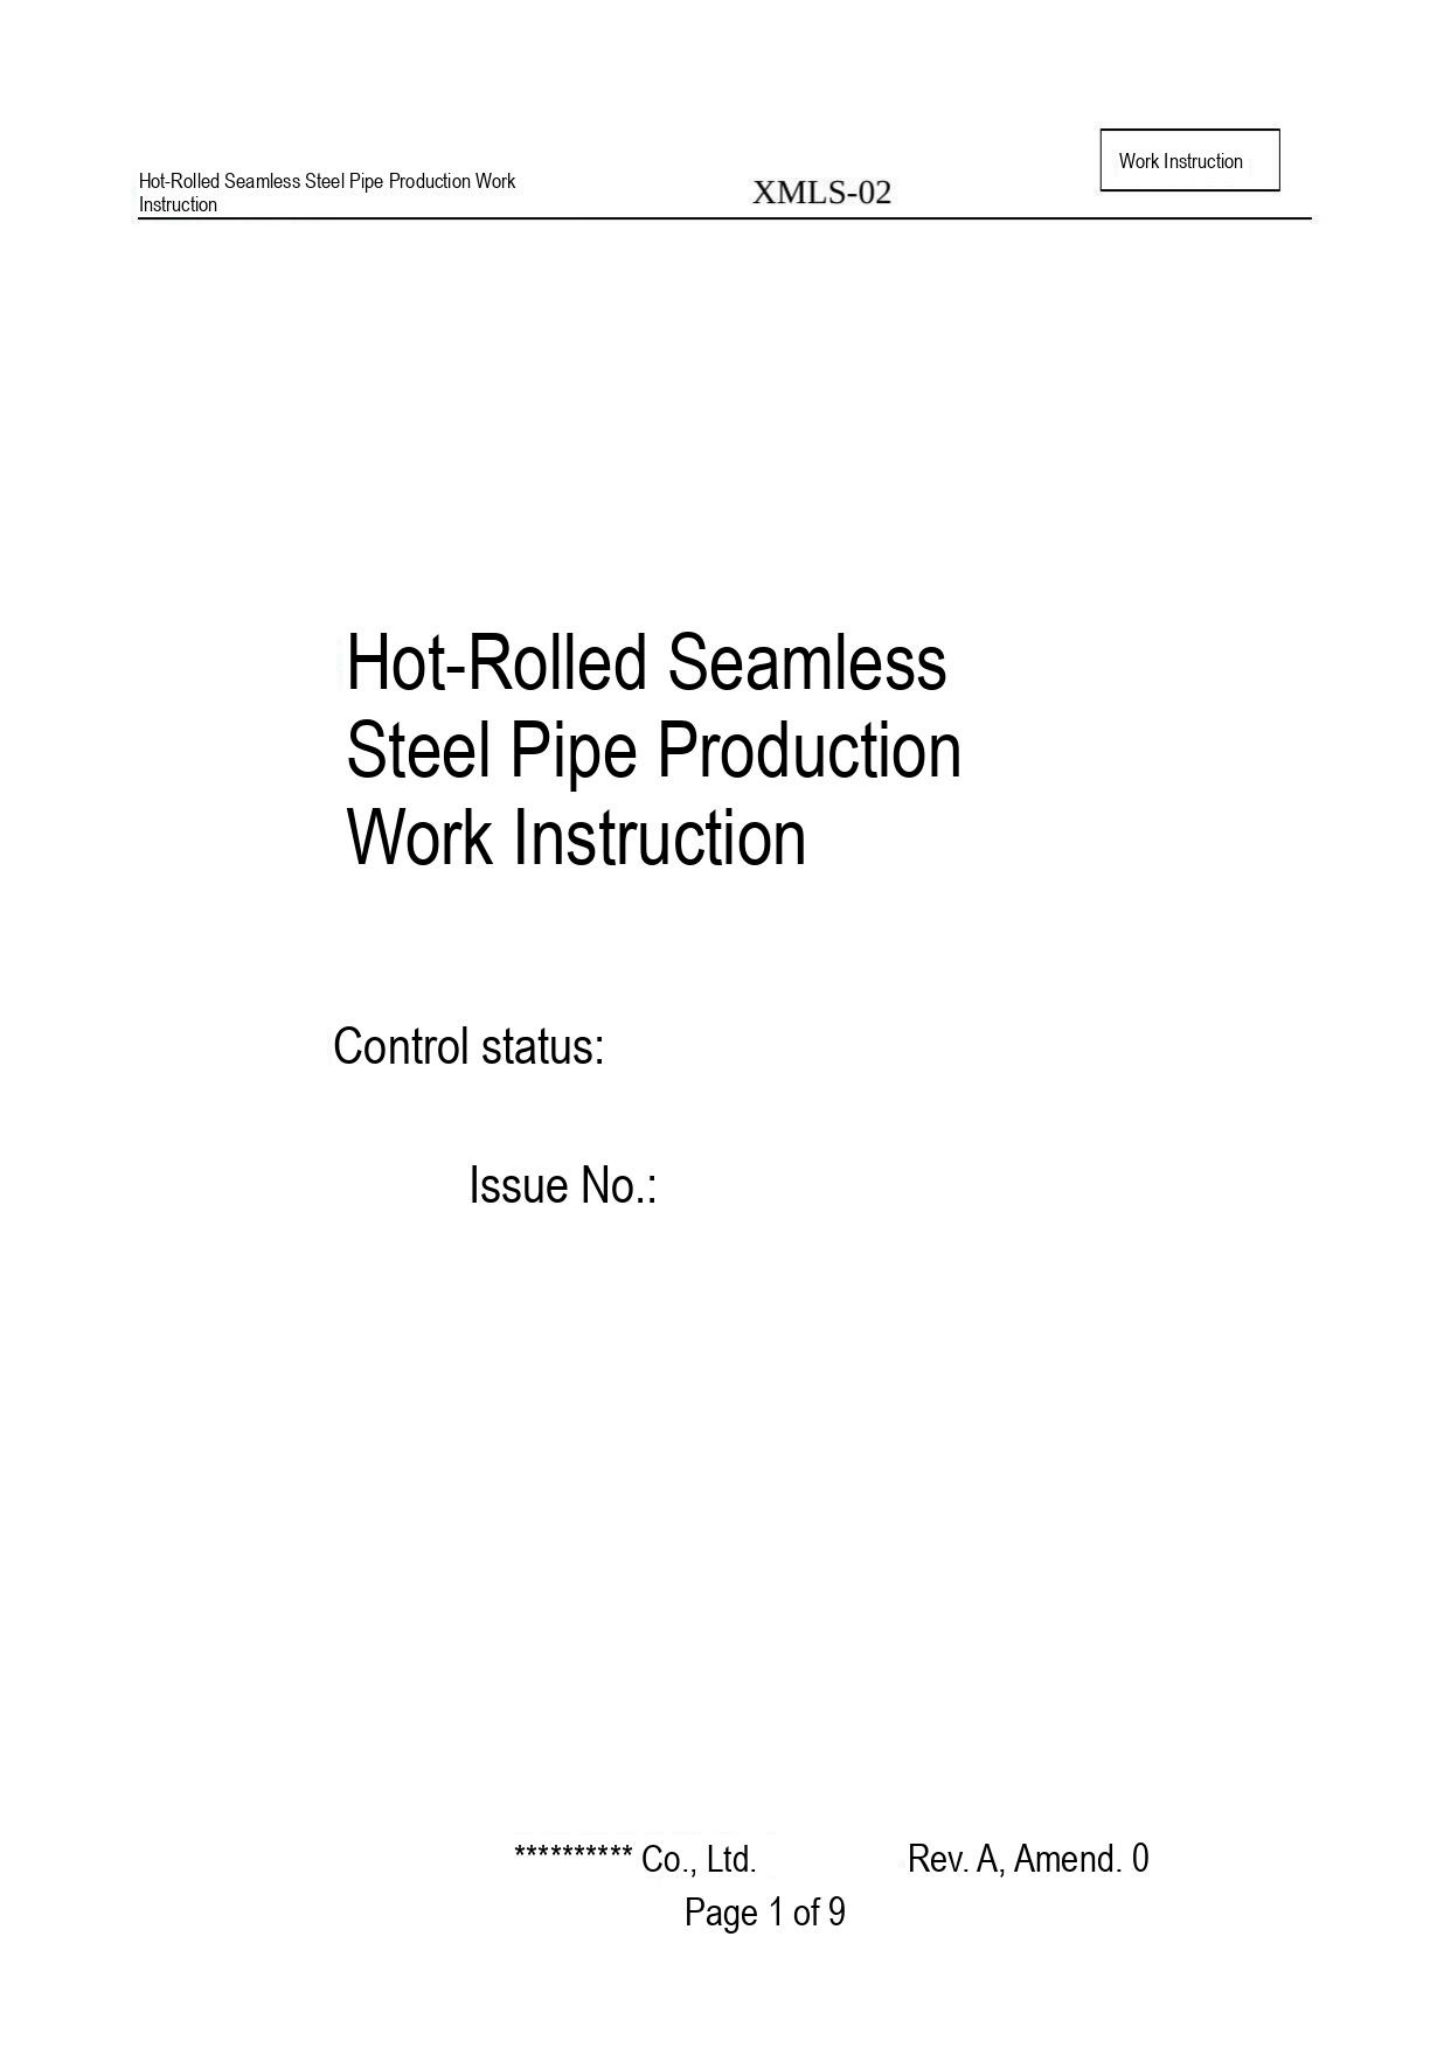Hot-Rolled Seamless Steel Pipe Production Work Instruction

XMLS-02

Work Instruction

Hot-Rolled Seamless Steel Pipe Production Work Instruction

Control status:

Issue No.:

********** Co., Ltd.

Rev. A, Amend. 0

Page 1 of 9
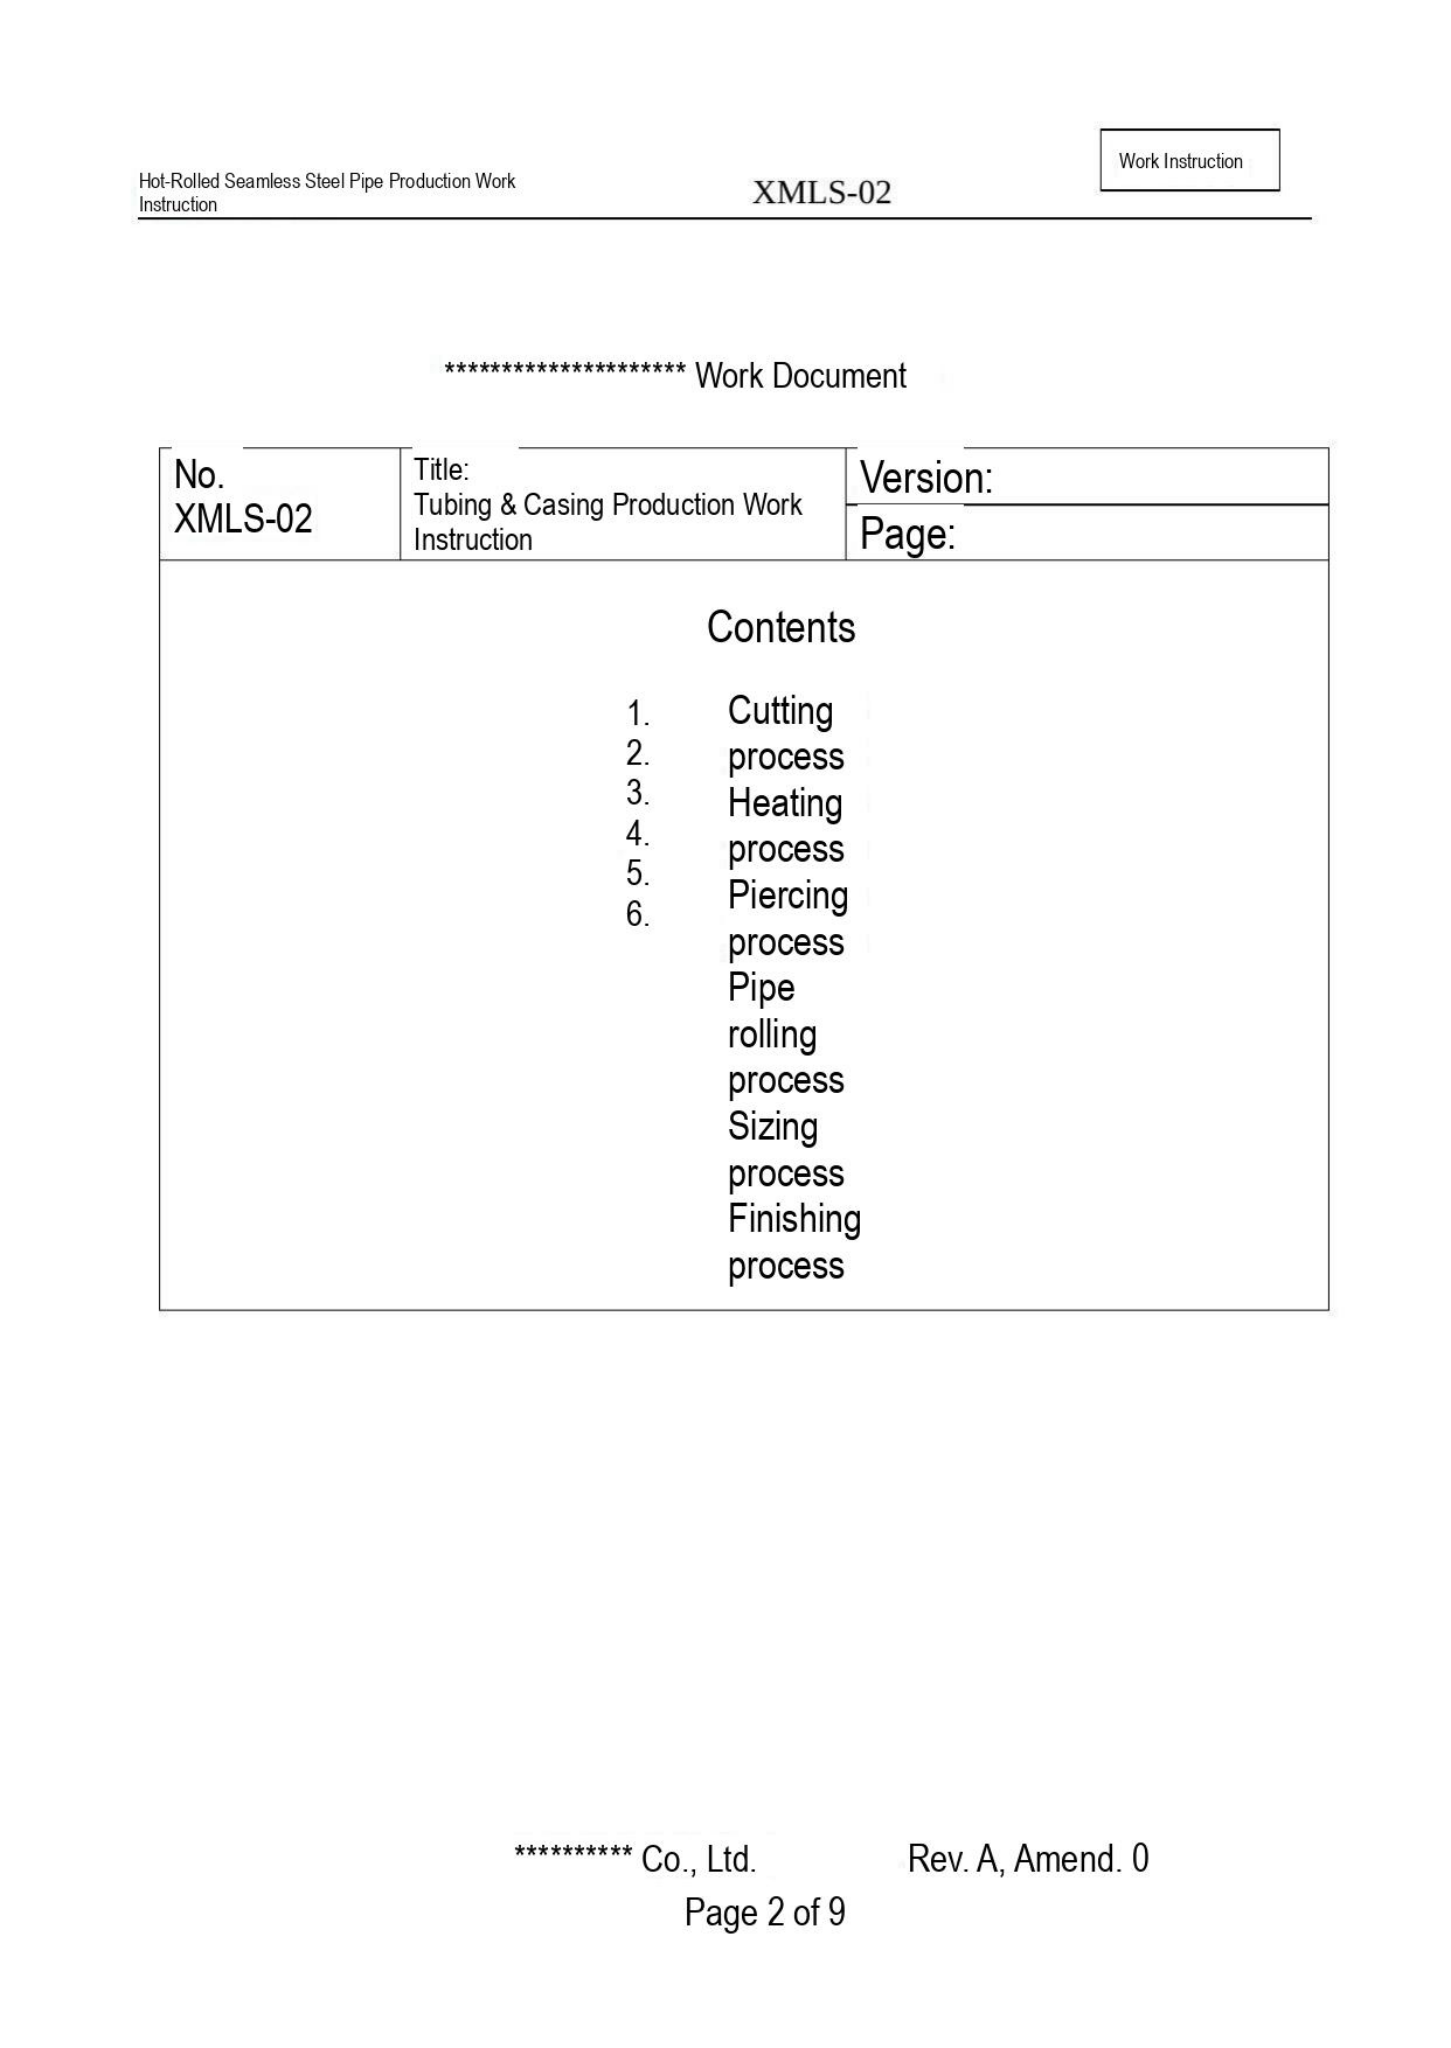Hot-Rolled Seamless Steel Pipe Production Work Instruction

XMLS-02

Work Instruction

********************* Work Document

| No. XMLS-02 | Title: Tubing & Casing Production Work Instruction | Version: |
|---|---|---|
| | | Page: |

Contents

1. Cutting process
2. Heating process
3. Piercing process
4. Pipe rolling process
5. Sizing process
6. Finishing process

********** Co., Ltd. Rev. A, Amend. 0

Page 2 of 9
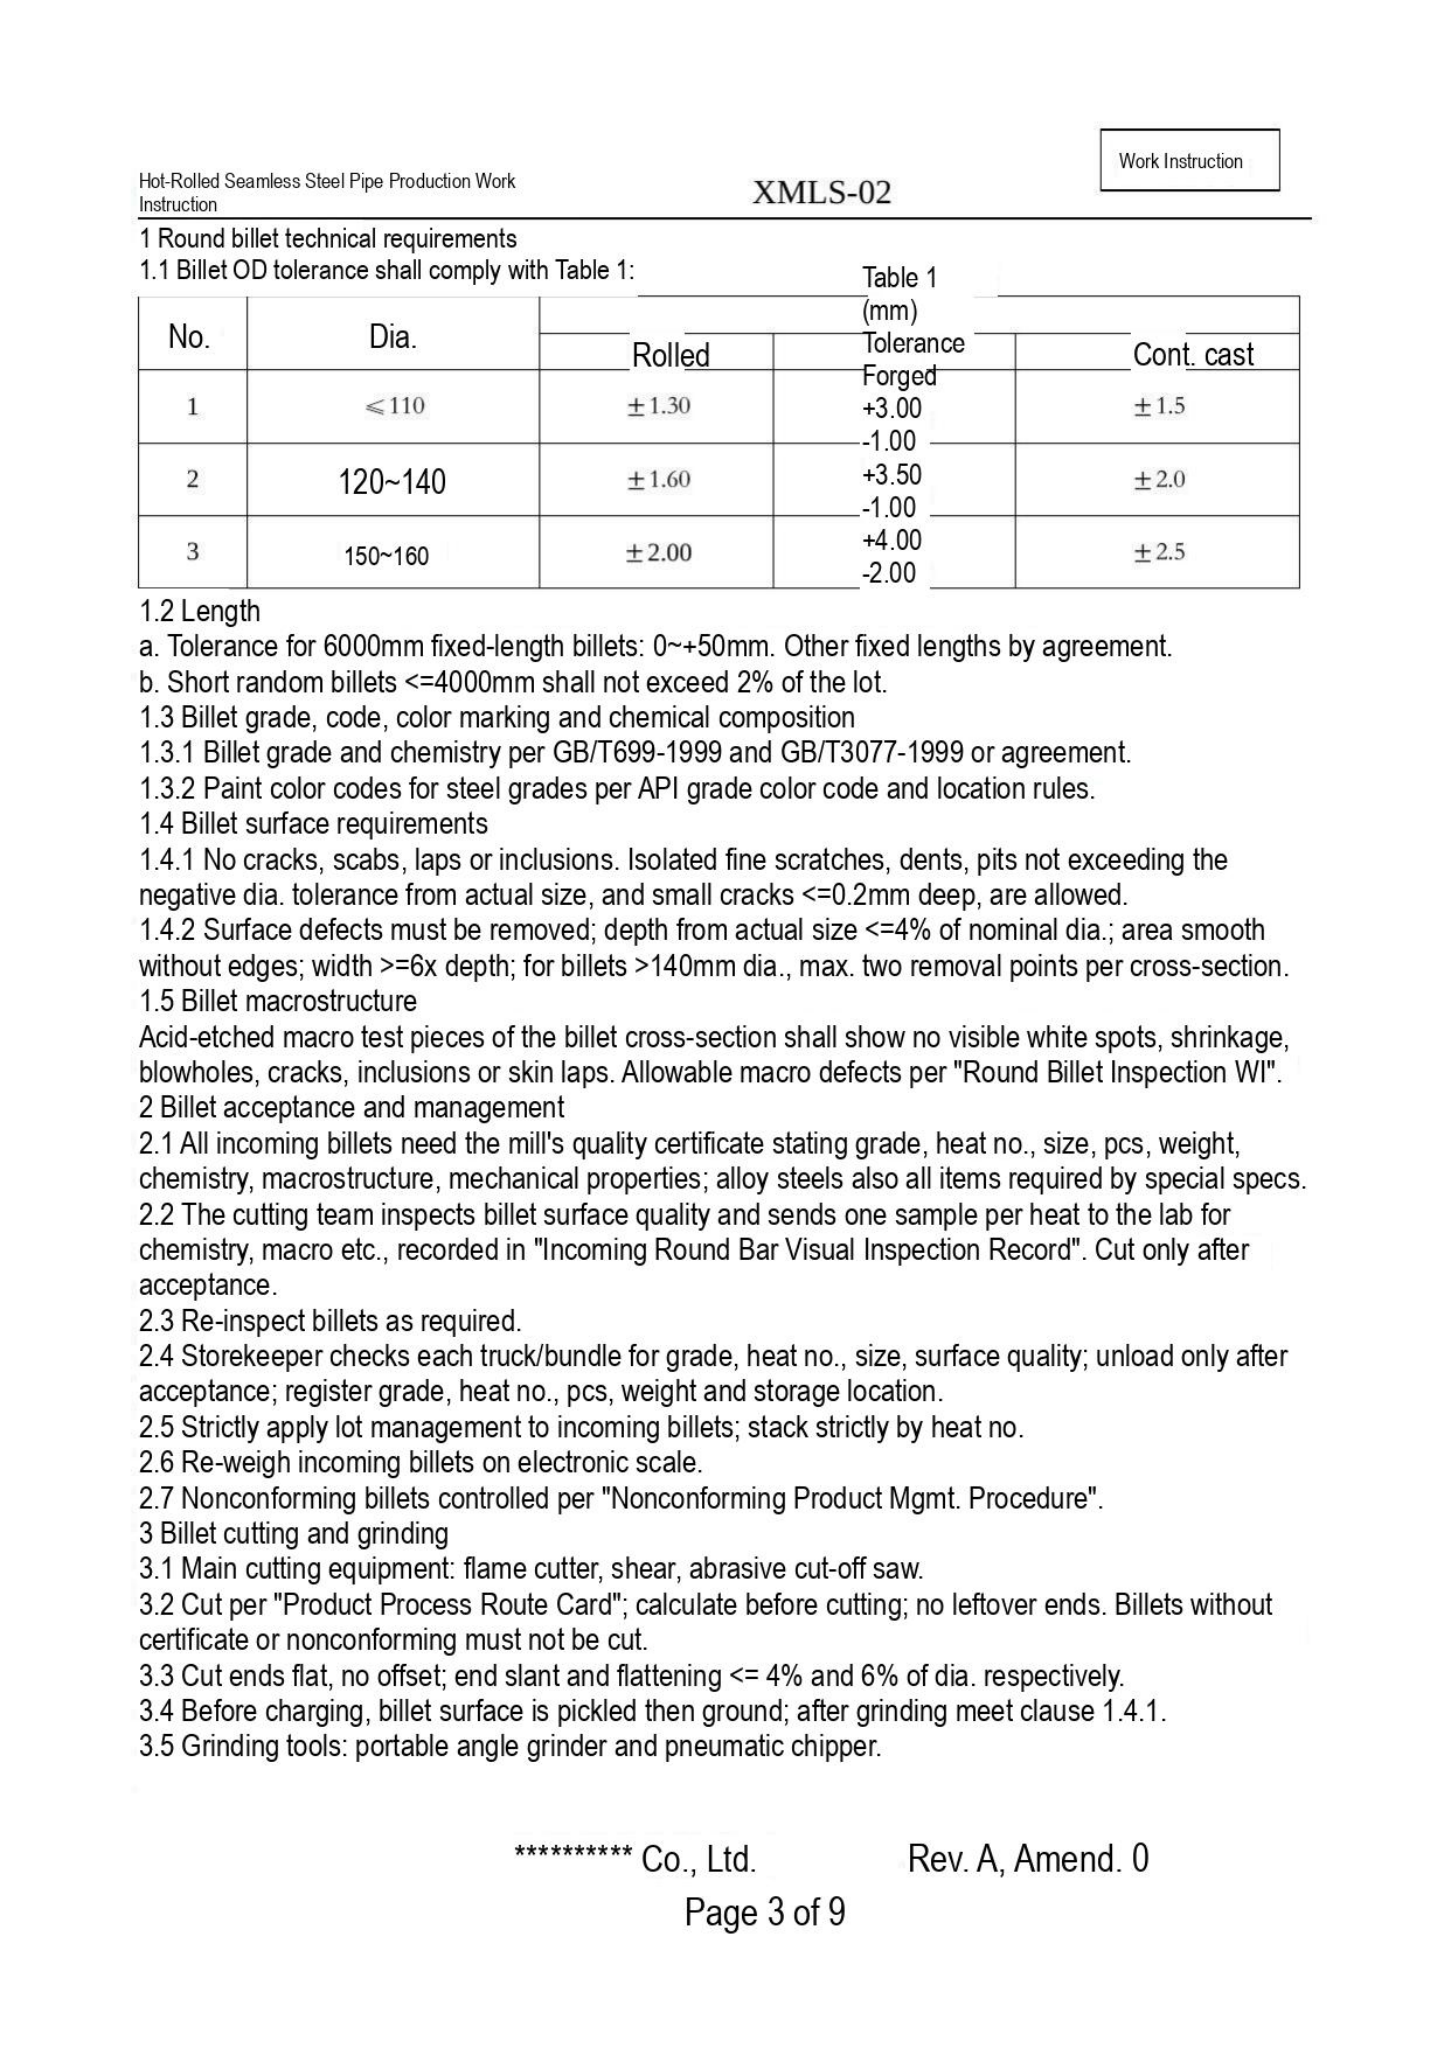Hot-Rolled Seamless Steel Pipe Production Work Instruction

XMLS-02

Work Instruction

1 Round billet technical requirements

1.1 Billet OD tolerance shall comply with Table 1:

Table 1 (mm)

| No. | Dia. | Tolerance<br>Rolled | Tolerance<br>Forged | Tolerance<br>Cont. cast |
|---|---|---|---|---|
| 1 | ≤110 | ±1.30 | +3.00<br>-1.00 | ±1.5 |
| 2 | 120~140 | ±1.60 | +3.50<br>-1.00 | ±2.0 |
| 3 | 150~160 | ±2.00 | +4.00<br>-2.00 | ±2.5 |

1.2 Length

a. Tolerance for 6000mm fixed-length billets: 0~+50mm. Other fixed lengths by agreement.

b. Short random billets <=4000mm shall not exceed 2% of the lot.

1.3 Billet grade, code, color marking and chemical composition

1.3.1 Billet grade and chemistry per GB/T699-1999 and GB/T3077-1999 or agreement.

1.3.2 Paint color codes for steel grades per API grade color code and location rules.

1.4 Billet surface requirements

1.4.1 No cracks, scabs, laps or inclusions. Isolated fine scratches, dents, pits not exceeding the negative dia. tolerance from actual size, and small cracks <=0.2mm deep, are allowed.

1.4.2 Surface defects must be removed; depth from actual size <=4% of nominal dia.; area smooth without edges; width >=6x depth; for billets >140mm dia., max. two removal points per cross-section.

1.5 Billet macrostructure

Acid-etched macro test pieces of the billet cross-section shall show no visible white spots, shrinkage, blowholes, cracks, inclusions or skin laps. Allowable macro defects per "Round Billet Inspection WI".

2 Billet acceptance and management

2.1 All incoming billets need the mill's quality certificate stating grade, heat no., size, pcs, weight, chemistry, macrostructure, mechanical properties; alloy steels also all items required by special specs.

2.2 The cutting team inspects billet surface quality and sends one sample per heat to the lab for chemistry, macro etc., recorded in "Incoming Round Bar Visual Inspection Record". Cut only after acceptance.

2.3 Re-inspect billets as required.

2.4 Storekeeper checks each truck/bundle for grade, heat no., size, surface quality; unload only after acceptance; register grade, heat no., pcs, weight and storage location.

2.5 Strictly apply lot management to incoming billets; stack strictly by heat no.

2.6 Re-weigh incoming billets on electronic scale.

2.7 Nonconforming billets controlled per "Nonconforming Product Mgmt. Procedure".

3 Billet cutting and grinding

3.1 Main cutting equipment: flame cutter, shear, abrasive cut-off saw.

3.2 Cut per "Product Process Route Card"; calculate before cutting; no leftover ends. Billets without certificate or nonconforming must not be cut.

3.3 Cut ends flat, no offset; end slant and flattening <= 4% and 6% of dia. respectively.

3.4 Before charging, billet surface is pickled then ground; after grinding meet clause 1.4.1.

3.5 Grinding tools: portable angle grinder and pneumatic chipper.

********** Co., Ltd. Rev. A, Amend. 0

Page 3 of 9
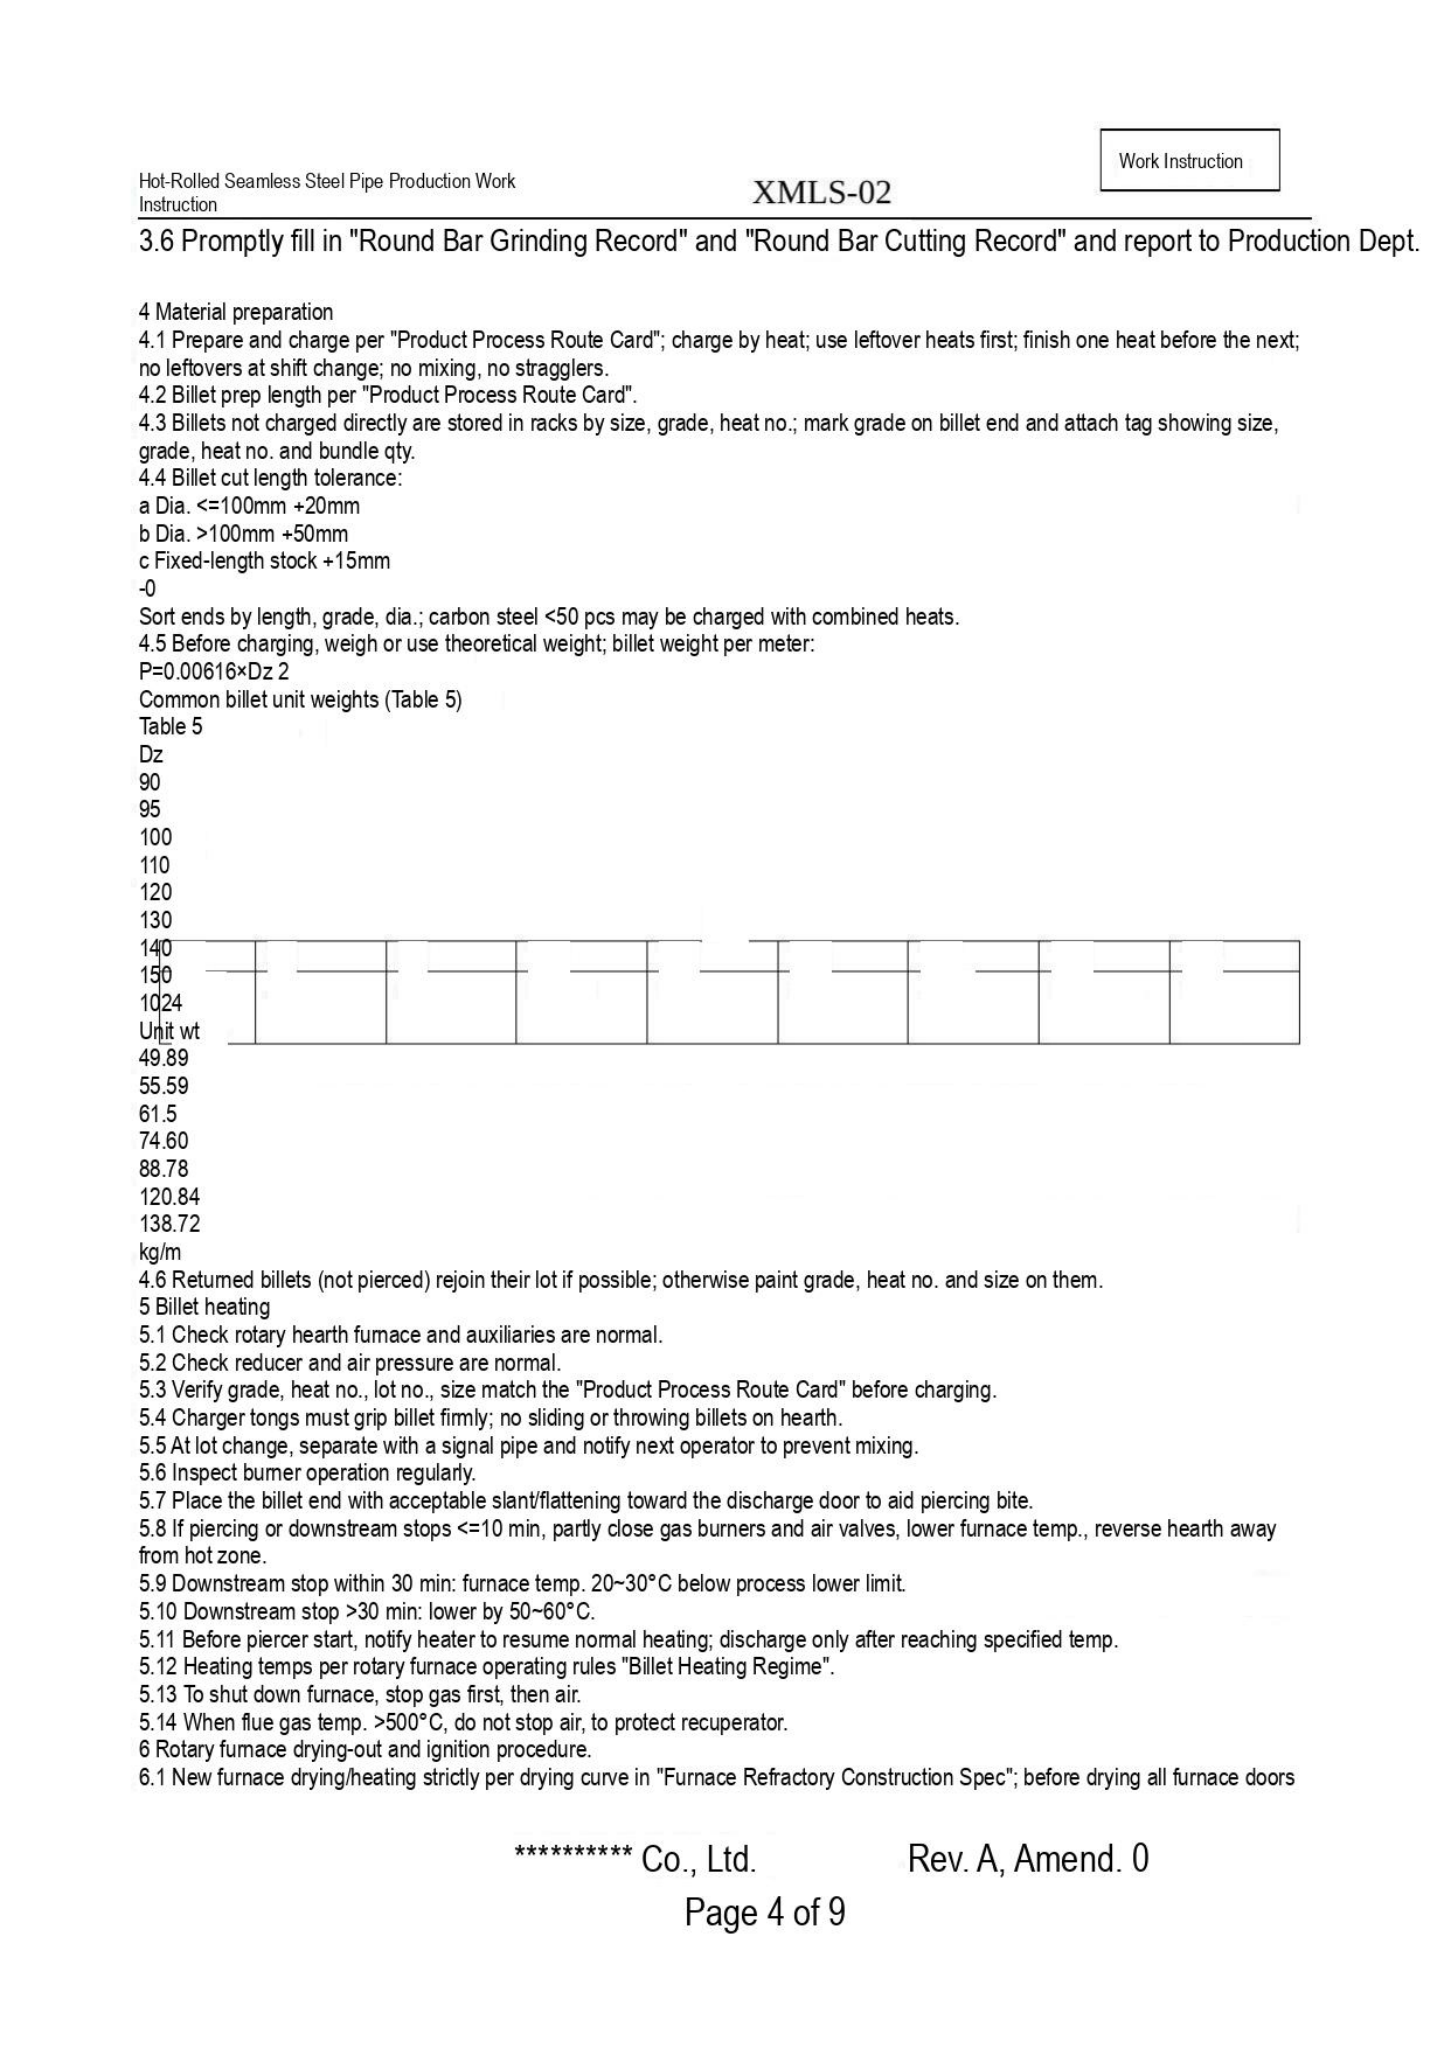Hot-Rolled Seamless Steel Pipe Production Work Instruction

XMLS-02

Work Instruction

3.6 Promptly fill in "Round Bar Grinding Record" and "Round Bar Cutting Record" and report to Production Dept.

4 Material preparation
4.1 Prepare and charge per "Product Process Route Card"; charge by heat; use leftover heats first; finish one heat before the next; no leftovers at shift change; no mixing, no stragglers.
4.2 Billet prep length per "Product Process Route Card".
4.3 Billets not charged directly are stored in racks by size, grade, heat no.; mark grade on billet end and attach tag showing size, grade, heat no. and bundle qty.
4.4 Billet cut length tolerance:
a Dia. <=100mm +20mm
b Dia. >100mm +50mm
c Fixed-length stock +15mm
-0
Sort ends by length, grade, dia.; carbon steel <50 pcs may be charged with combined heats.
4.5 Before charging, weigh or use theoretical weight; billet weight per meter:
P=0.00616×Dz 2
Common billet unit weights (Table 5)
Table 5
Dz
90
95
100
110
120
130
140
150
1024
Unit wt
49.89
55.59
61.5
74.60
88.78
120.84
138.72
kg/m
4.6 Returned billets (not pierced) rejoin their lot if possible; otherwise paint grade, heat no. and size on them.
5 Billet heating
5.1 Check rotary hearth furnace and auxiliaries are normal.
5.2 Check reducer and air pressure are normal.
5.3 Verify grade, heat no., lot no., size match the "Product Process Route Card" before charging.
5.4 Charger tongs must grip billet firmly; no sliding or throwing billets on hearth.
5.5 At lot change, separate with a signal pipe and notify next operator to prevent mixing.
5.6 Inspect burner operation regularly.
5.7 Place the billet end with acceptable slant/flattening toward the discharge door to aid piercing bite.
5.8 If piercing or downstream stops <=10 min, partly close gas burners and air valves, lower furnace temp., reverse hearth away from hot zone.
5.9 Downstream stop within 30 min: furnace temp. 20~30°C below process lower limit.
5.10 Downstream stop >30 min: lower by 50~60°C.
5.11 Before piercer start, notify heater to resume normal heating; discharge only after reaching specified temp.
5.12 Heating temps per rotary furnace operating rules "Billet Heating Regime".
5.13 To shut down furnace, stop gas first, then air.
5.14 When flue gas temp. >500°C, do not stop air, to protect recuperator.
6 Rotary furnace drying-out and ignition procedure.
6.1 New furnace drying/heating strictly per drying curve in "Furnace Refractory Construction Spec"; before drying all furnace doors

********** Co., Ltd. Rev. A, Amend. 0

Page 4 of 9
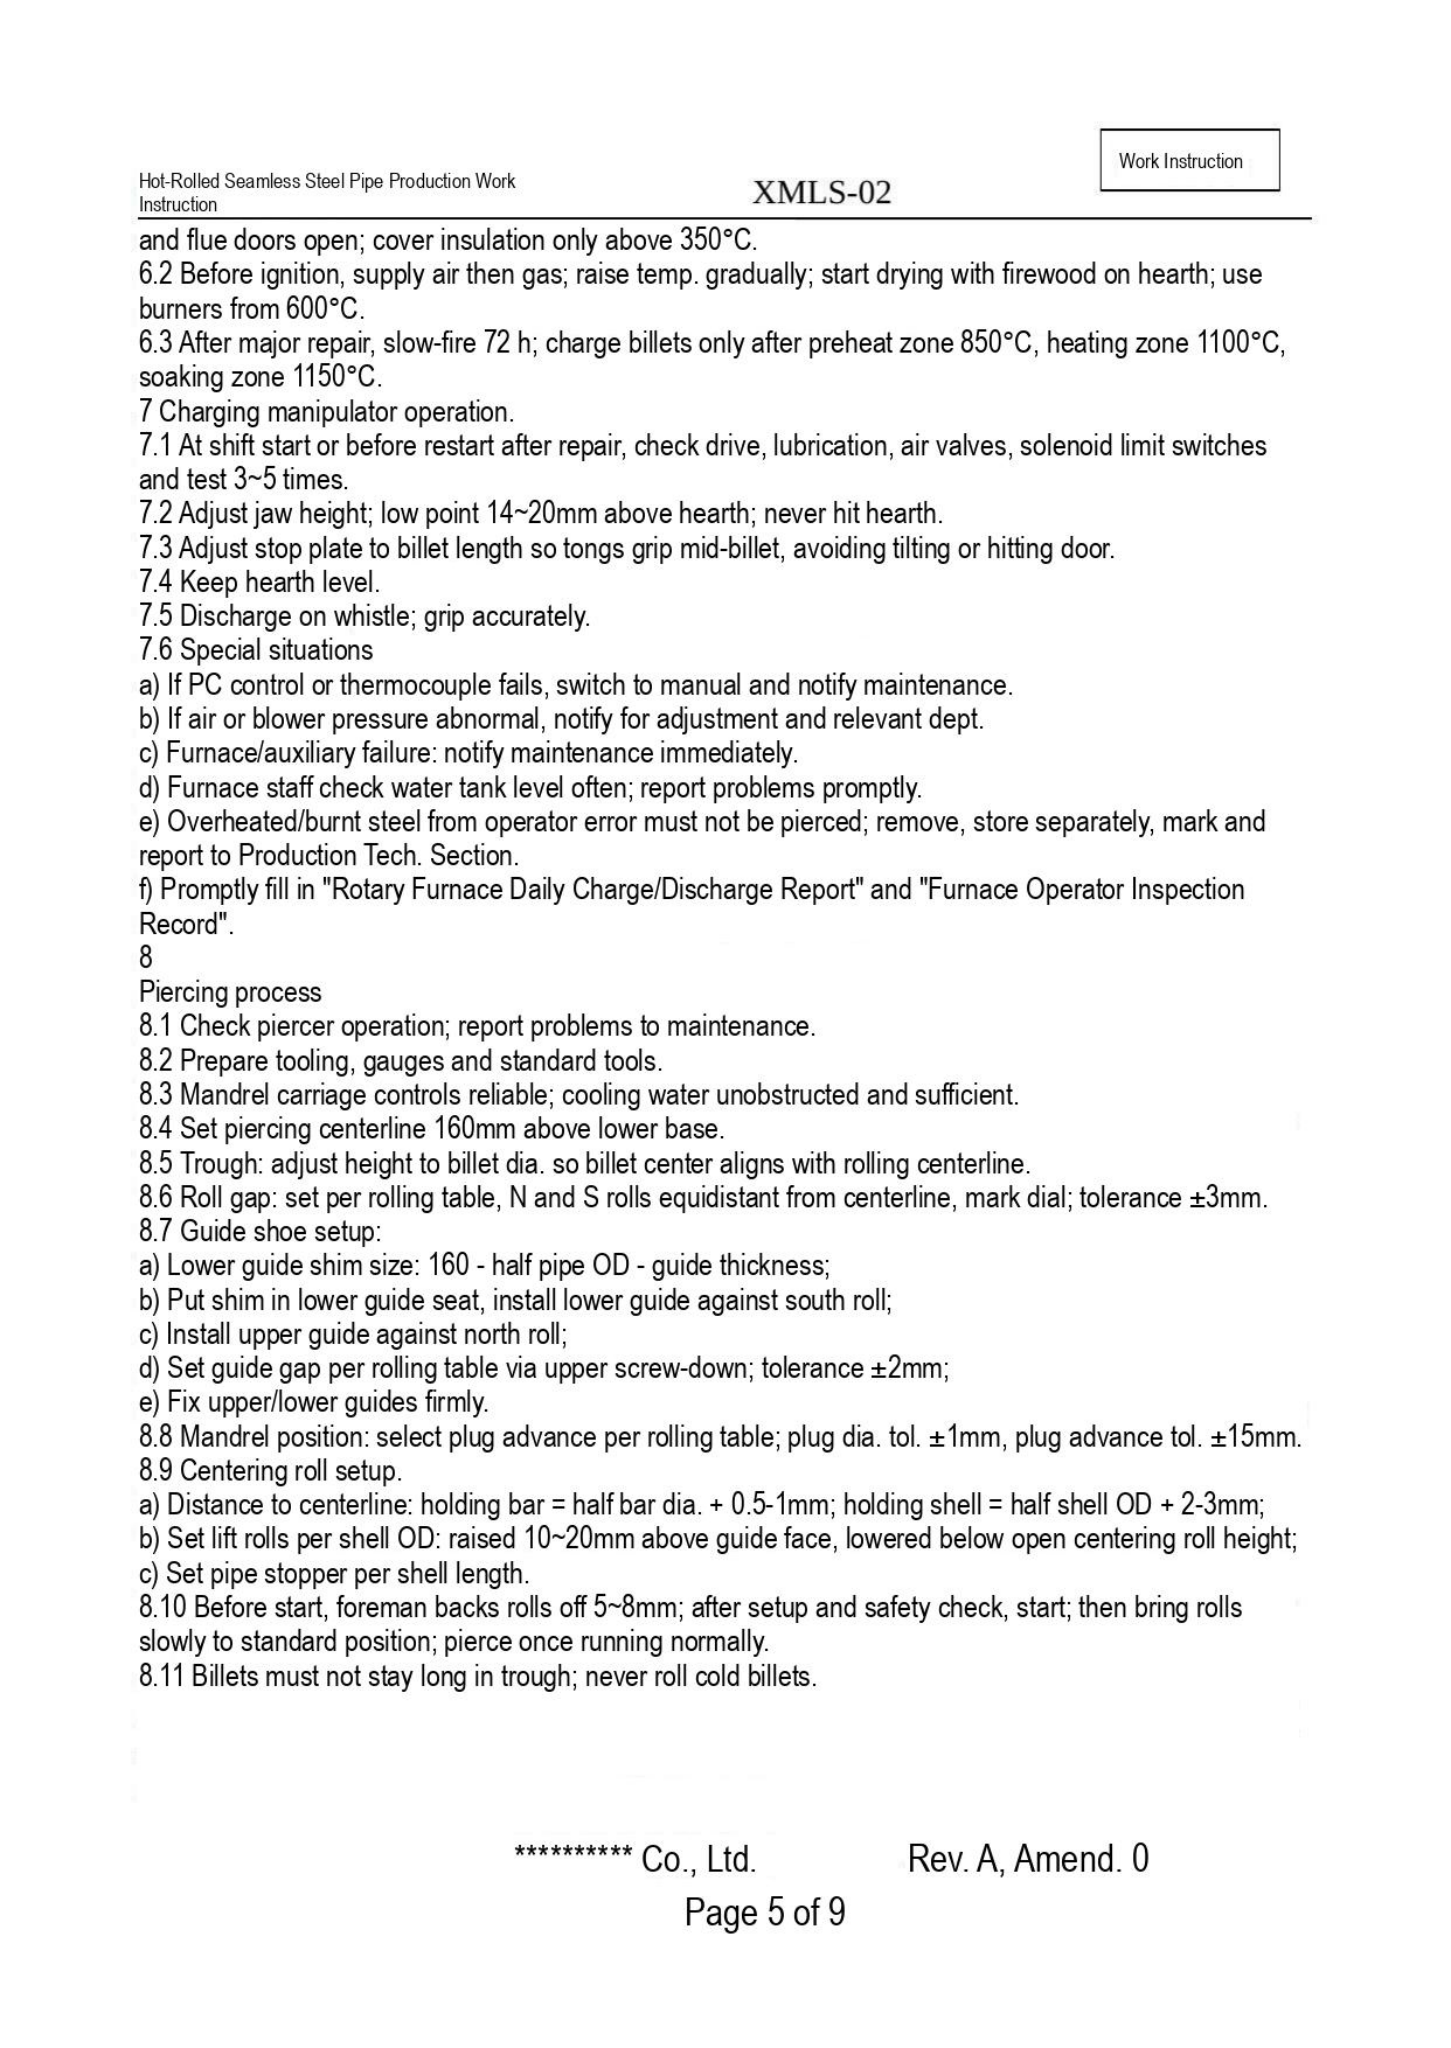Hot-Rolled Seamless Steel Pipe Production Work Instruction

XMLS-02

Work Instruction

and flue doors open; cover insulation only above 350°C.
6.2 Before ignition, supply air then gas; raise temp. gradually; start drying with firewood on hearth; use burners from 600°C.
6.3 After major repair, slow-fire 72 h; charge billets only after preheat zone 850°C, heating zone 1100°C, soaking zone 1150°C.
7 Charging manipulator operation.
7.1 At shift start or before restart after repair, check drive, lubrication, air valves, solenoid limit switches and test 3~5 times.
7.2 Adjust jaw height; low point 14~20mm above hearth; never hit hearth.
7.3 Adjust stop plate to billet length so tongs grip mid-billet, avoiding tilting or hitting door.
7.4 Keep hearth level.
7.5 Discharge on whistle; grip accurately.
7.6 Special situations
a) If PC control or thermocouple fails, switch to manual and notify maintenance.
b) If air or blower pressure abnormal, notify for adjustment and relevant dept.
c) Furnace/auxiliary failure: notify maintenance immediately.
d) Furnace staff check water tank level often; report problems promptly.
e) Overheated/burnt steel from operator error must not be pierced; remove, store separately, mark and report to Production Tech. Section.
f) Promptly fill in "Rotary Furnace Daily Charge/Discharge Report" and "Furnace Operator Inspection Record".
8
Piercing process
8.1 Check piercer operation; report problems to maintenance.
8.2 Prepare tooling, gauges and standard tools.
8.3 Mandrel carriage controls reliable; cooling water unobstructed and sufficient.
8.4 Set piercing centerline 160mm above lower base.
8.5 Trough: adjust height to billet dia. so billet center aligns with rolling centerline.
8.6 Roll gap: set per rolling table, N and S rolls equidistant from centerline, mark dial; tolerance ±3mm.
8.7 Guide shoe setup:
a) Lower guide shim size: 160 - half pipe OD - guide thickness;
b) Put shim in lower guide seat, install lower guide against south roll;
c) Install upper guide against north roll;
d) Set guide gap per rolling table via upper screw-down; tolerance ±2mm;
e) Fix upper/lower guides firmly.
8.8 Mandrel position: select plug advance per rolling table; plug dia. tol. ±1mm, plug advance tol. ±15mm.
8.9 Centering roll setup.
a) Distance to centerline: holding bar = half bar dia. + 0.5-1mm; holding shell = half shell OD + 2-3mm;
b) Set lift rolls per shell OD: raised 10~20mm above guide face, lowered below open centering roll height;
c) Set pipe stopper per shell length.
8.10 Before start, foreman backs rolls off 5~8mm; after setup and safety check, start; then bring rolls slowly to standard position; pierce once running normally.
8.11 Billets must not stay long in trough; never roll cold billets.

********** Co., Ltd. Rev. A, Amend. 0

Page 5 of 9
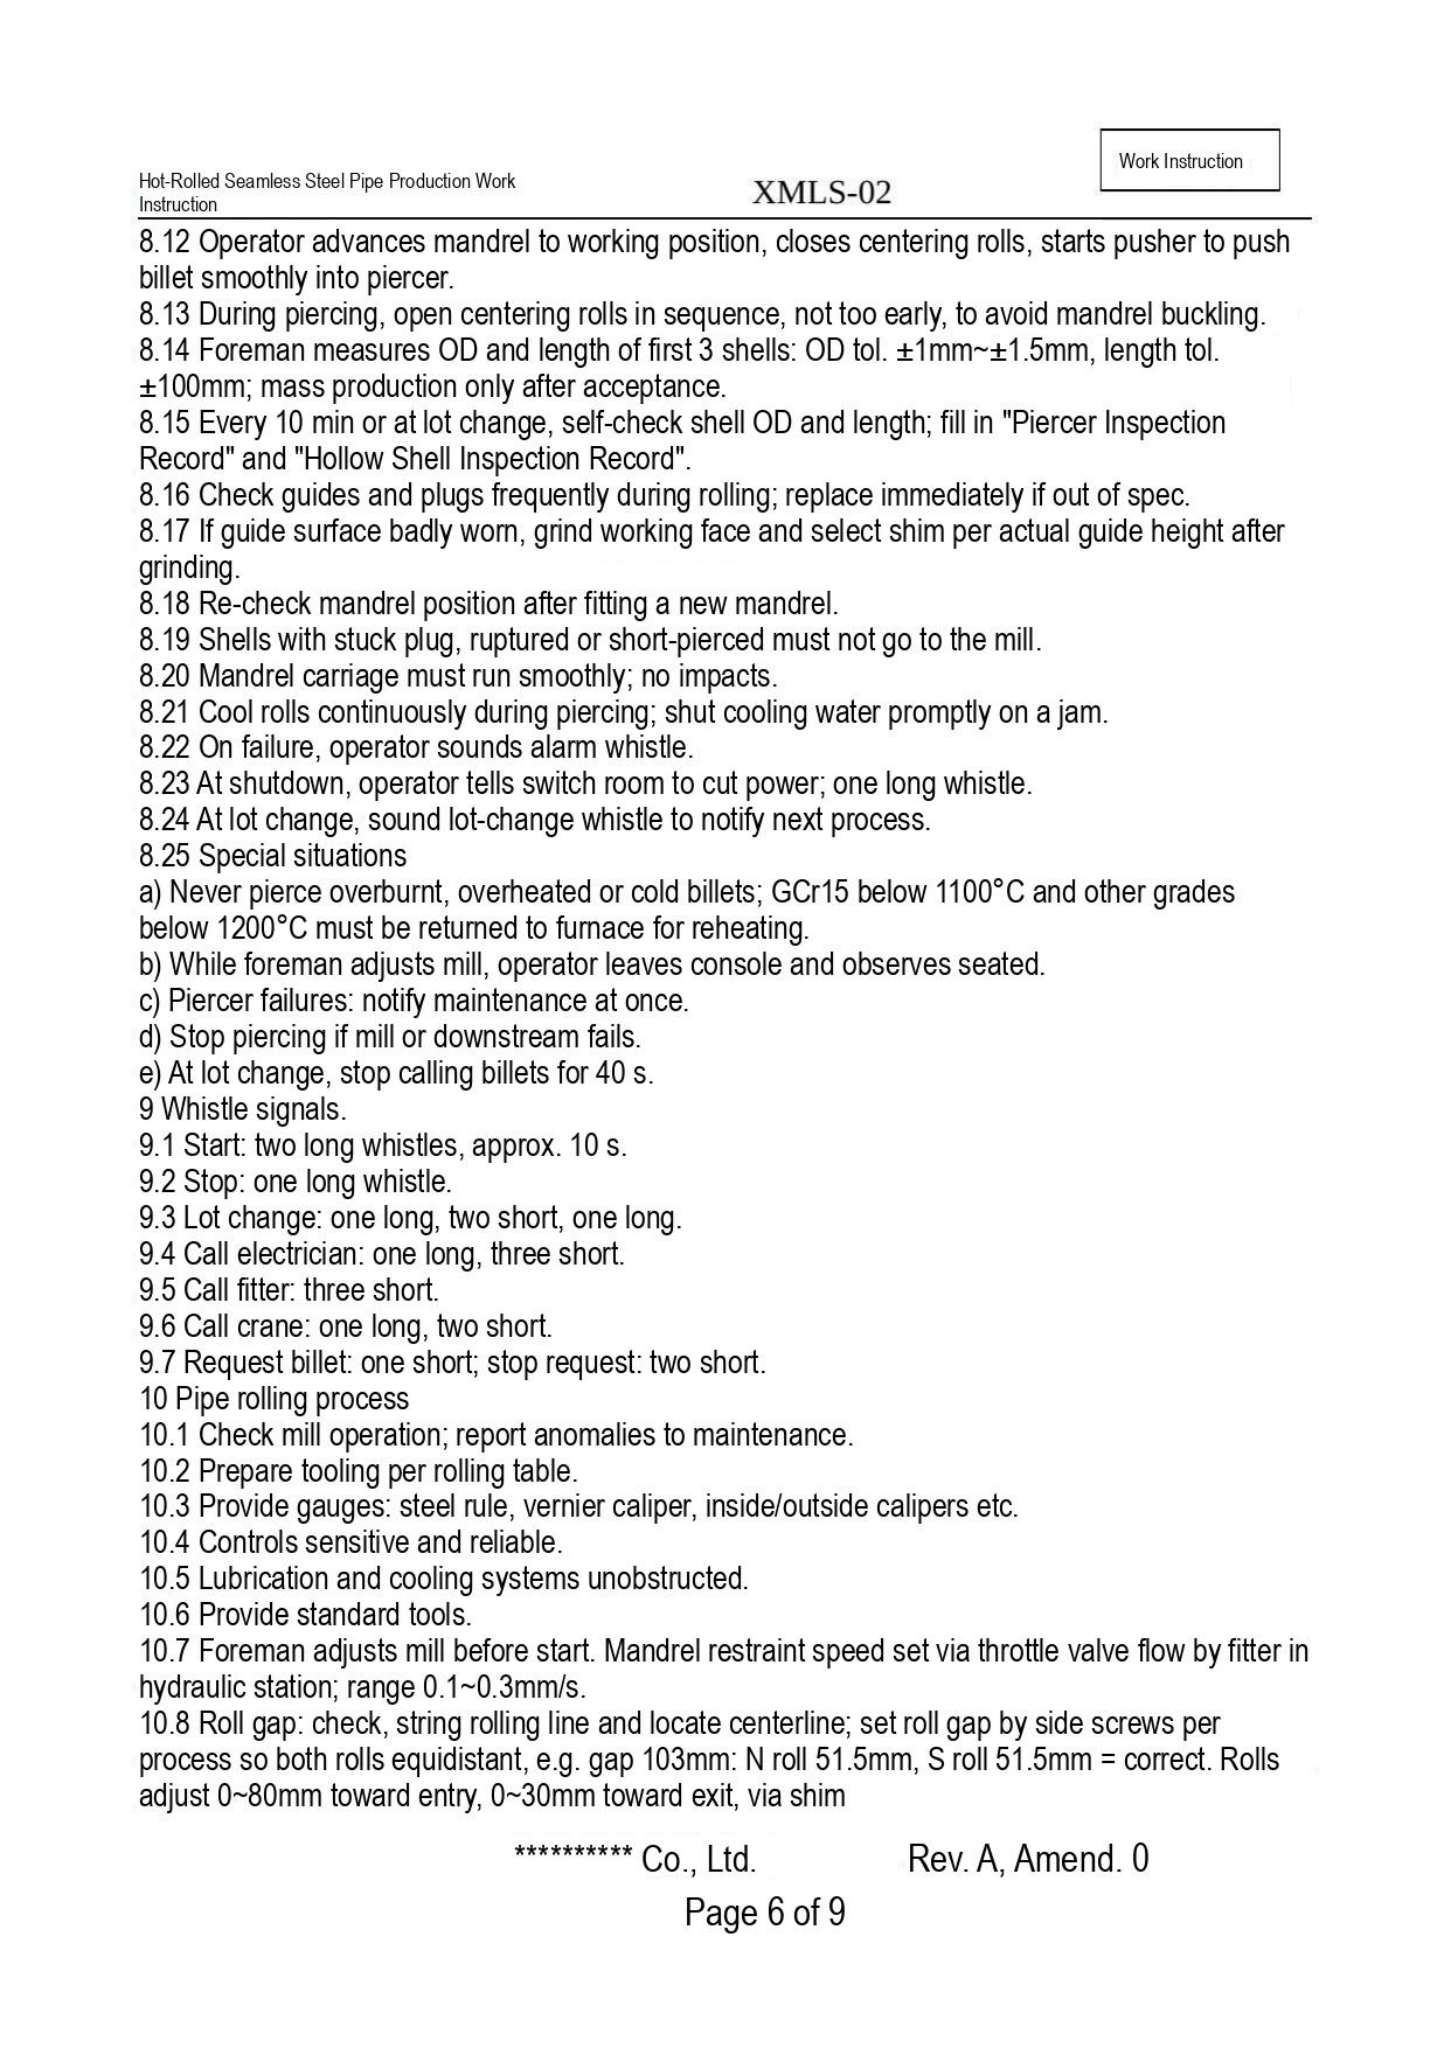Hot-Rolled Seamless Steel Pipe Production Work Instruction XMLS-02 Work Instruction

8.12 Operator advances mandrel to working position, closes centering rolls, starts pusher to push billet smoothly into piercer.
8.13 During piercing, open centering rolls in sequence, not too early, to avoid mandrel buckling.
8.14 Foreman measures OD and length of first 3 shells: OD tol. ±1mm~±1.5mm, length tol. ±100mm; mass production only after acceptance.
8.15 Every 10 min or at lot change, self-check shell OD and length; fill in "Piercer Inspection Record" and "Hollow Shell Inspection Record".
8.16 Check guides and plugs frequently during rolling; replace immediately if out of spec.
8.17 If guide surface badly worn, grind working face and select shim per actual guide height after grinding.
8.18 Re-check mandrel position after fitting a new mandrel.
8.19 Shells with stuck plug, ruptured or short-pierced must not go to the mill.
8.20 Mandrel carriage must run smoothly; no impacts.
8.21 Cool rolls continuously during piercing; shut cooling water promptly on a jam.
8.22 On failure, operator sounds alarm whistle.
8.23 At shutdown, operator tells switch room to cut power; one long whistle.
8.24 At lot change, sound lot-change whistle to notify next process.
8.25 Special situations
a) Never pierce overburnt, overheated or cold billets; GCr15 below 1100°C and other grades below 1200°C must be returned to furnace for reheating.
b) While foreman adjusts mill, operator leaves console and observes seated.
c) Piercer failures: notify maintenance at once.
d) Stop piercing if mill or downstream fails.
e) At lot change, stop calling billets for 40 s.
9 Whistle signals.
9.1 Start: two long whistles, approx. 10 s.
9.2 Stop: one long whistle.
9.3 Lot change: one long, two short, one long.
9.4 Call electrician: one long, three short.
9.5 Call fitter: three short.
9.6 Call crane: one long, two short.
9.7 Request billet: one short; stop request: two short.
10 Pipe rolling process
10.1 Check mill operation; report anomalies to maintenance.
10.2 Prepare tooling per rolling table.
10.3 Provide gauges: steel rule, vernier caliper, inside/outside calipers etc.
10.4 Controls sensitive and reliable.
10.5 Lubrication and cooling systems unobstructed.
10.6 Provide standard tools.
10.7 Foreman adjusts mill before start. Mandrel restraint speed set via throttle valve flow by fitter in hydraulic station; range 0.1~0.3mm/s.
10.8 Roll gap: check, string rolling line and locate centerline; set roll gap by side screws per process so both rolls equidistant, e.g. gap 103mm: N roll 51.5mm, S roll 51.5mm = correct. Rolls adjust 0~80mm toward entry, 0~30mm toward exit, via shim

********** Co., Ltd. Rev. A, Amend. 0

Page 6 of 9